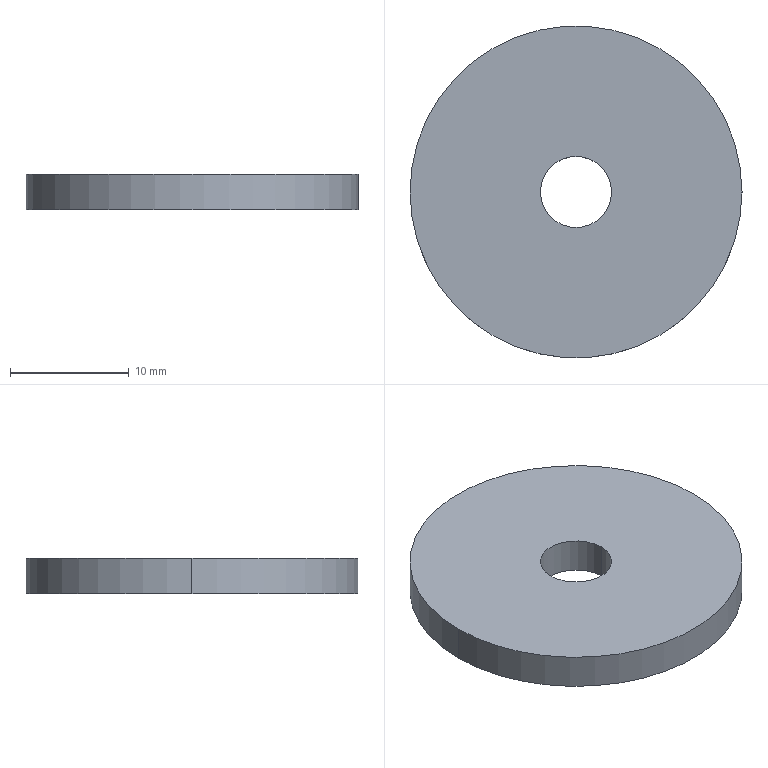Part | SolidWorks | features Extrusion 1 | 1 solid | 6 faces | box 28 x 28 x 3 mm | volume 1762 mm3 | cylinder 4 | plane 2 | commonest cylinder face diameters 6 x2 28 x2
STEP:
#1=CARTESIAN_POINT('',(-3.,0.,3.));
#2=VERTEX_POINT('',#1);
#3=CARTESIAN_POINT('',(3.,0.,3.));
#4=VERTEX_POINT('',#3);
#5=CARTESIAN_POINT('',(0.,0.,3.));
#6=DIRECTION('',(0.,0.,1.));
#7=DIRECTION('',(1.,0.,0.));
#8=AXIS2_PLACEMENT_3D('',#5,#6,#7);
#9=CIRCLE('',#8,3.);
#10=EDGE_CURVE('',#2,#4,#9,.T.);
#11=ORIENTED_EDGE('',*,*,#10,.T.);
#12=CARTESIAN_POINT('',(3.,0.,0.));
#13=VERTEX_POINT('',#12);
#14=CARTESIAN_POINT('',(3.,0.,3.));
#15=DIRECTION('',(0.,0.,-1.));
#16=VECTOR('',#15,1000.);
#17=LINE('',#14,#16);
#18=EDGE_CURVE('',#4,#13,#17,.T.);
#19=ORIENTED_EDGE('',*,*,#18,.T.);
#20=CARTESIAN_POINT('',(-3.,0.,0.));
#21=VERTEX_POINT('',#20);
#22=CARTESIAN_POINT('',(0.,0.,0.));
#23=DIRECTION('',(0.,0.,1.));
#24=DIRECTION('',(1.,0.,0.));
#25=AXIS2_PLACEMENT_3D('',#22,#23,#24);
#26=CIRCLE('',#25,3.);
#27=EDGE_CURVE('',#21,#13,#26,.T.);
#28=ORIENTED_EDGE('',*,*,#27,.F.);
#29=CARTESIAN_POINT('',(-3.,0.,3.));
#30=DIRECTION('',(0.,0.,-1.));
#31=VECTOR('',#30,1000.);
#32=LINE('',#29,#31);
#33=EDGE_CURVE('',#2,#21,#32,.T.);
#34=ORIENTED_EDGE('',*,*,#33,.F.);
#35=EDGE_LOOP('',(#11,#19,#28,#34));
#36=FACE_OUTER_BOUND('',#35,.T.);
#37=CARTESIAN_POINT('',(0.,0.,3.));
#38=DIRECTION('',(0.,0.,-1.));
#39=DIRECTION('',(-1.,0.,0.));
#40=AXIS2_PLACEMENT_3D('',#37,#38,#39);
#41=CYLINDRICAL_SURFACE('',#40,3.);
#42=ADVANCED_FACE('',(#36),#41,.F.);
#43=CARTESIAN_POINT('',(14.,0.,3.));
#44=VERTEX_POINT('',#43);
#45=CARTESIAN_POINT('',(-14.,0.,3.));
#46=VERTEX_POINT('',#45);
#47=CARTESIAN_POINT('',(0.,0.,3.));
#48=DIRECTION('',(0.,0.,1.));
#49=DIRECTION('',(1.,0.,0.));
#50=AXIS2_PLACEMENT_3D('',#47,#48,#49);
#51=CIRCLE('',#50,14.);
#52=EDGE_CURVE('',#44,#46,#51,.T.);
#53=ORIENTED_EDGE('',*,*,#52,.F.);
#54=CARTESIAN_POINT('',(14.,0.,0.));
#55=VERTEX_POINT('',#54);
#56=CARTESIAN_POINT('',(14.,0.,3.));
#57=DIRECTION('',(0.,0.,-1.));
#58=VECTOR('',#57,1000.);
#59=LINE('',#56,#58);
#60=EDGE_CURVE('',#44,#55,#59,.T.);
#61=ORIENTED_EDGE('',*,*,#60,.T.);
#62=CARTESIAN_POINT('',(-14.,0.,0.));
#63=VERTEX_POINT('',#62);
#64=CARTESIAN_POINT('',(0.,0.,0.));
#65=DIRECTION('',(0.,0.,1.));
#66=DIRECTION('',(1.,0.,0.));
#67=AXIS2_PLACEMENT_3D('',#64,#65,#66);
#68=CIRCLE('',#67,14.);
#69=EDGE_CURVE('',#55,#63,#68,.T.);
#70=ORIENTED_EDGE('',*,*,#69,.T.);
#71=CARTESIAN_POINT('',(-14.,0.,3.));
#72=DIRECTION('',(0.,0.,-1.));
#73=VECTOR('',#72,1000.);
#74=LINE('',#71,#73);
#75=EDGE_CURVE('',#46,#63,#74,.T.);
#76=ORIENTED_EDGE('',*,*,#75,.F.);
#77=EDGE_LOOP('',(#53,#61,#70,#76));
#78=FACE_OUTER_BOUND('',#77,.T.);
#79=CARTESIAN_POINT('',(0.,0.,3.));
#80=DIRECTION('',(0.,0.,-1.));
#81=DIRECTION('',(-1.,0.,0.));
#82=AXIS2_PLACEMENT_3D('',#79,#80,#81);
#83=CYLINDRICAL_SURFACE('',#82,14.);
#84=ADVANCED_FACE('',(#78),#83,.T.);
#85=CARTESIAN_POINT('',(0.,0.,3.));
#86=DIRECTION('',(0.,0.,1.));
#87=DIRECTION('',(1.,0.,0.));
#88=AXIS2_PLACEMENT_3D('',#85,#86,#87);
#89=CIRCLE('',#88,14.);
#90=EDGE_CURVE('',#46,#44,#89,.T.);
#91=ORIENTED_EDGE('',*,*,#90,.T.);
#92=ORIENTED_EDGE('',*,*,#52,.T.);
#93=EDGE_LOOP('',(#91,#92));
#94=FACE_OUTER_BOUND('',#93,.T.);
#95=ORIENTED_EDGE('',*,*,#10,.F.);
#96=CARTESIAN_POINT('',(0.,0.,3.));
#97=DIRECTION('',(0.,0.,1.));
#98=DIRECTION('',(1.,0.,0.));
#99=AXIS2_PLACEMENT_3D('',#96,#97,#98);
#100=CIRCLE('',#99,3.);
#101=EDGE_CURVE('',#4,#2,#100,.T.);
#102=ORIENTED_EDGE('',*,*,#101,.F.);
#103=EDGE_LOOP('',(#95,#102));
#104=FACE_BOUND('',#103,.T.);
#105=CARTESIAN_POINT('',(0.,0.,3.));
#106=DIRECTION('',(0.,0.,1.));
#107=DIRECTION('',(1.,0.,0.));
#108=AXIS2_PLACEMENT_3D('',#105,#106,#107);
#109=PLANE('',#108);
#110=ADVANCED_FACE('',(#94,#104),#109,.T.);
#111=CARTESIAN_POINT('',(0.,0.,0.));
#112=DIRECTION('',(0.,0.,1.));
#113=DIRECTION('',(1.,0.,0.));
#114=AXIS2_PLACEMENT_3D('',#111,#112,#113);
#115=CIRCLE('',#114,14.);
#116=EDGE_CURVE('',#63,#55,#115,.T.);
#117=ORIENTED_EDGE('',*,*,#116,.F.);
#118=ORIENTED_EDGE('',*,*,#69,.F.);
#119=EDGE_LOOP('',(#117,#118));
#120=FACE_OUTER_BOUND('',#119,.T.);
#121=ORIENTED_EDGE('',*,*,#27,.T.);
#122=CARTESIAN_POINT('',(0.,0.,0.));
#123=DIRECTION('',(0.,0.,1.));
#124=DIRECTION('',(1.,0.,0.));
#125=AXIS2_PLACEMENT_3D('',#122,#123,#124);
#126=CIRCLE('',#125,3.);
#127=EDGE_CURVE('',#13,#21,#126,.T.);
#128=ORIENTED_EDGE('',*,*,#127,.T.);
#129=EDGE_LOOP('',(#121,#128));
#130=FACE_BOUND('',#129,.T.);
#131=CARTESIAN_POINT('',(0.,0.,0.));
#132=DIRECTION('',(0.,0.,1.));
#133=DIRECTION('',(1.,0.,0.));
#134=AXIS2_PLACEMENT_3D('',#131,#132,#133);
#135=PLANE('',#134);
#136=ADVANCED_FACE('',(#120,#130),#135,.F.);
#137=ORIENTED_EDGE('',*,*,#60,.F.);
#138=ORIENTED_EDGE('',*,*,#90,.F.);
#139=ORIENTED_EDGE('',*,*,#75,.T.);
#140=ORIENTED_EDGE('',*,*,#116,.T.);
#141=EDGE_LOOP('',(#137,#138,#139,#140));
#142=FACE_OUTER_BOUND('',#141,.T.);
#143=CARTESIAN_POINT('',(0.,0.,3.));
#144=DIRECTION('',(0.,0.,-1.));
#145=DIRECTION('',(-1.,0.,0.));
#146=AXIS2_PLACEMENT_3D('',#143,#144,#145);
#147=CYLINDRICAL_SURFACE('',#146,14.);
#148=ADVANCED_FACE('',(#142),#147,.T.);
#149=ORIENTED_EDGE('',*,*,#18,.F.);
#150=ORIENTED_EDGE('',*,*,#101,.T.);
#151=ORIENTED_EDGE('',*,*,#33,.T.);
#152=ORIENTED_EDGE('',*,*,#127,.F.);
#153=EDGE_LOOP('',(#149,#150,#151,#152));
#154=FACE_OUTER_BOUND('',#153,.T.);
#155=CARTESIAN_POINT('',(0.,0.,3.));
#156=DIRECTION('',(0.,0.,-1.));
#157=DIRECTION('',(-1.,0.,0.));
#158=AXIS2_PLACEMENT_3D('',#155,#156,#157);
#159=CYLINDRICAL_SURFACE('',#158,3.);
#160=ADVANCED_FACE('',(#154),#159,.F.);
#161=CLOSED_SHELL('',(#42,#84,#110,#136,#148,#160));
#162=MANIFOLD_SOLID_BREP('',#161);
#163=CARTESIAN_POINT('',(0.,0.,0.));
#164=DIRECTION('',(0.,0.,1.));
#165=DIRECTION('',(1.,0.,0.));
#166=AXIS2_PLACEMENT_3D('',#163,#164,#165);
#167=(LENGTH_UNIT()NAMED_UNIT(*)SI_UNIT(.MILLI.,.METRE.));
#168=UNCERTAINTY_MEASURE_WITH_UNIT(LENGTH_MEASURE(0.00001),#167,'','');
#169=(NAMED_UNIT(*)PLANE_ANGLE_UNIT()SI_UNIT($,.RADIAN.));
#170=(NAMED_UNIT(*)SI_UNIT($,.STERADIAN.)SOLID_ANGLE_UNIT());
#171=(GEOMETRIC_REPRESENTATION_CONTEXT(3)GLOBAL_UNCERTAINTY_ASSIGNED_CONTEXT((#168))GLOBAL_UNIT_ASSIGNED_CONTEXT((#167,#169,#170))REPRESENTATION_CONTEXT('',''));
#172=ADVANCED_BREP_SHAPE_REPRESENTATION('',(#162,#166),#171);